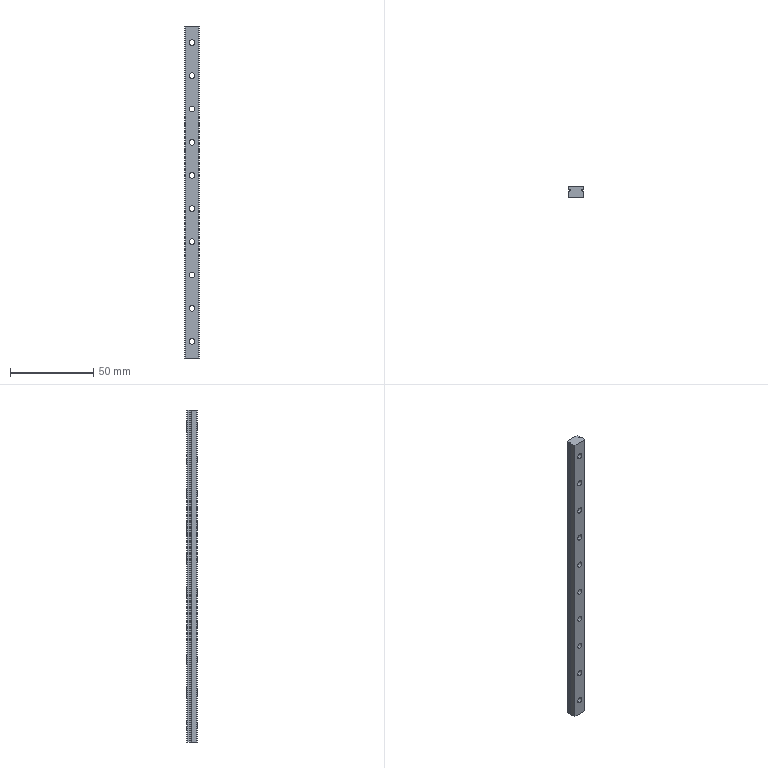Part | STEP file | 1 solid | 76 faces | box 9 x 6.5 x 200 mm | volume 10020 mm3 | cylinder 48 | plane 28 | commonest cylinder face diameters 3.5 x20 6 x20 0.18 x4 1.616 x4